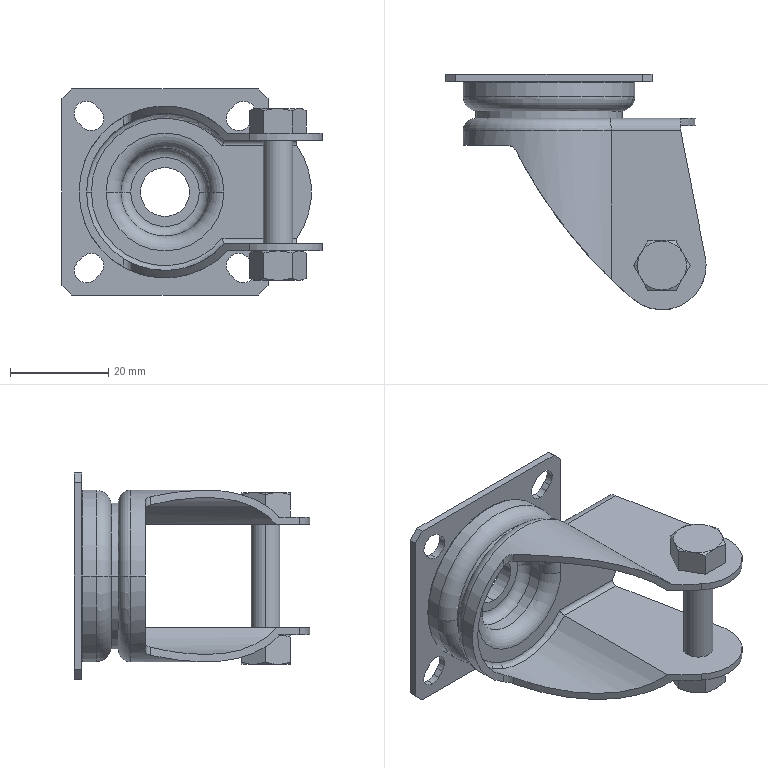Part | STEP file | PN_0001 Wheel body | 1 solid | 124 faces | box 53 x 48 x 42 mm | volume 13526 mm3 | plane 48 | cylinder 41 | cone 23 | torus 12 | commonest cylinder face diameters 5 x14 18 x6 6 x4 35 x4 2 x2 4 x2